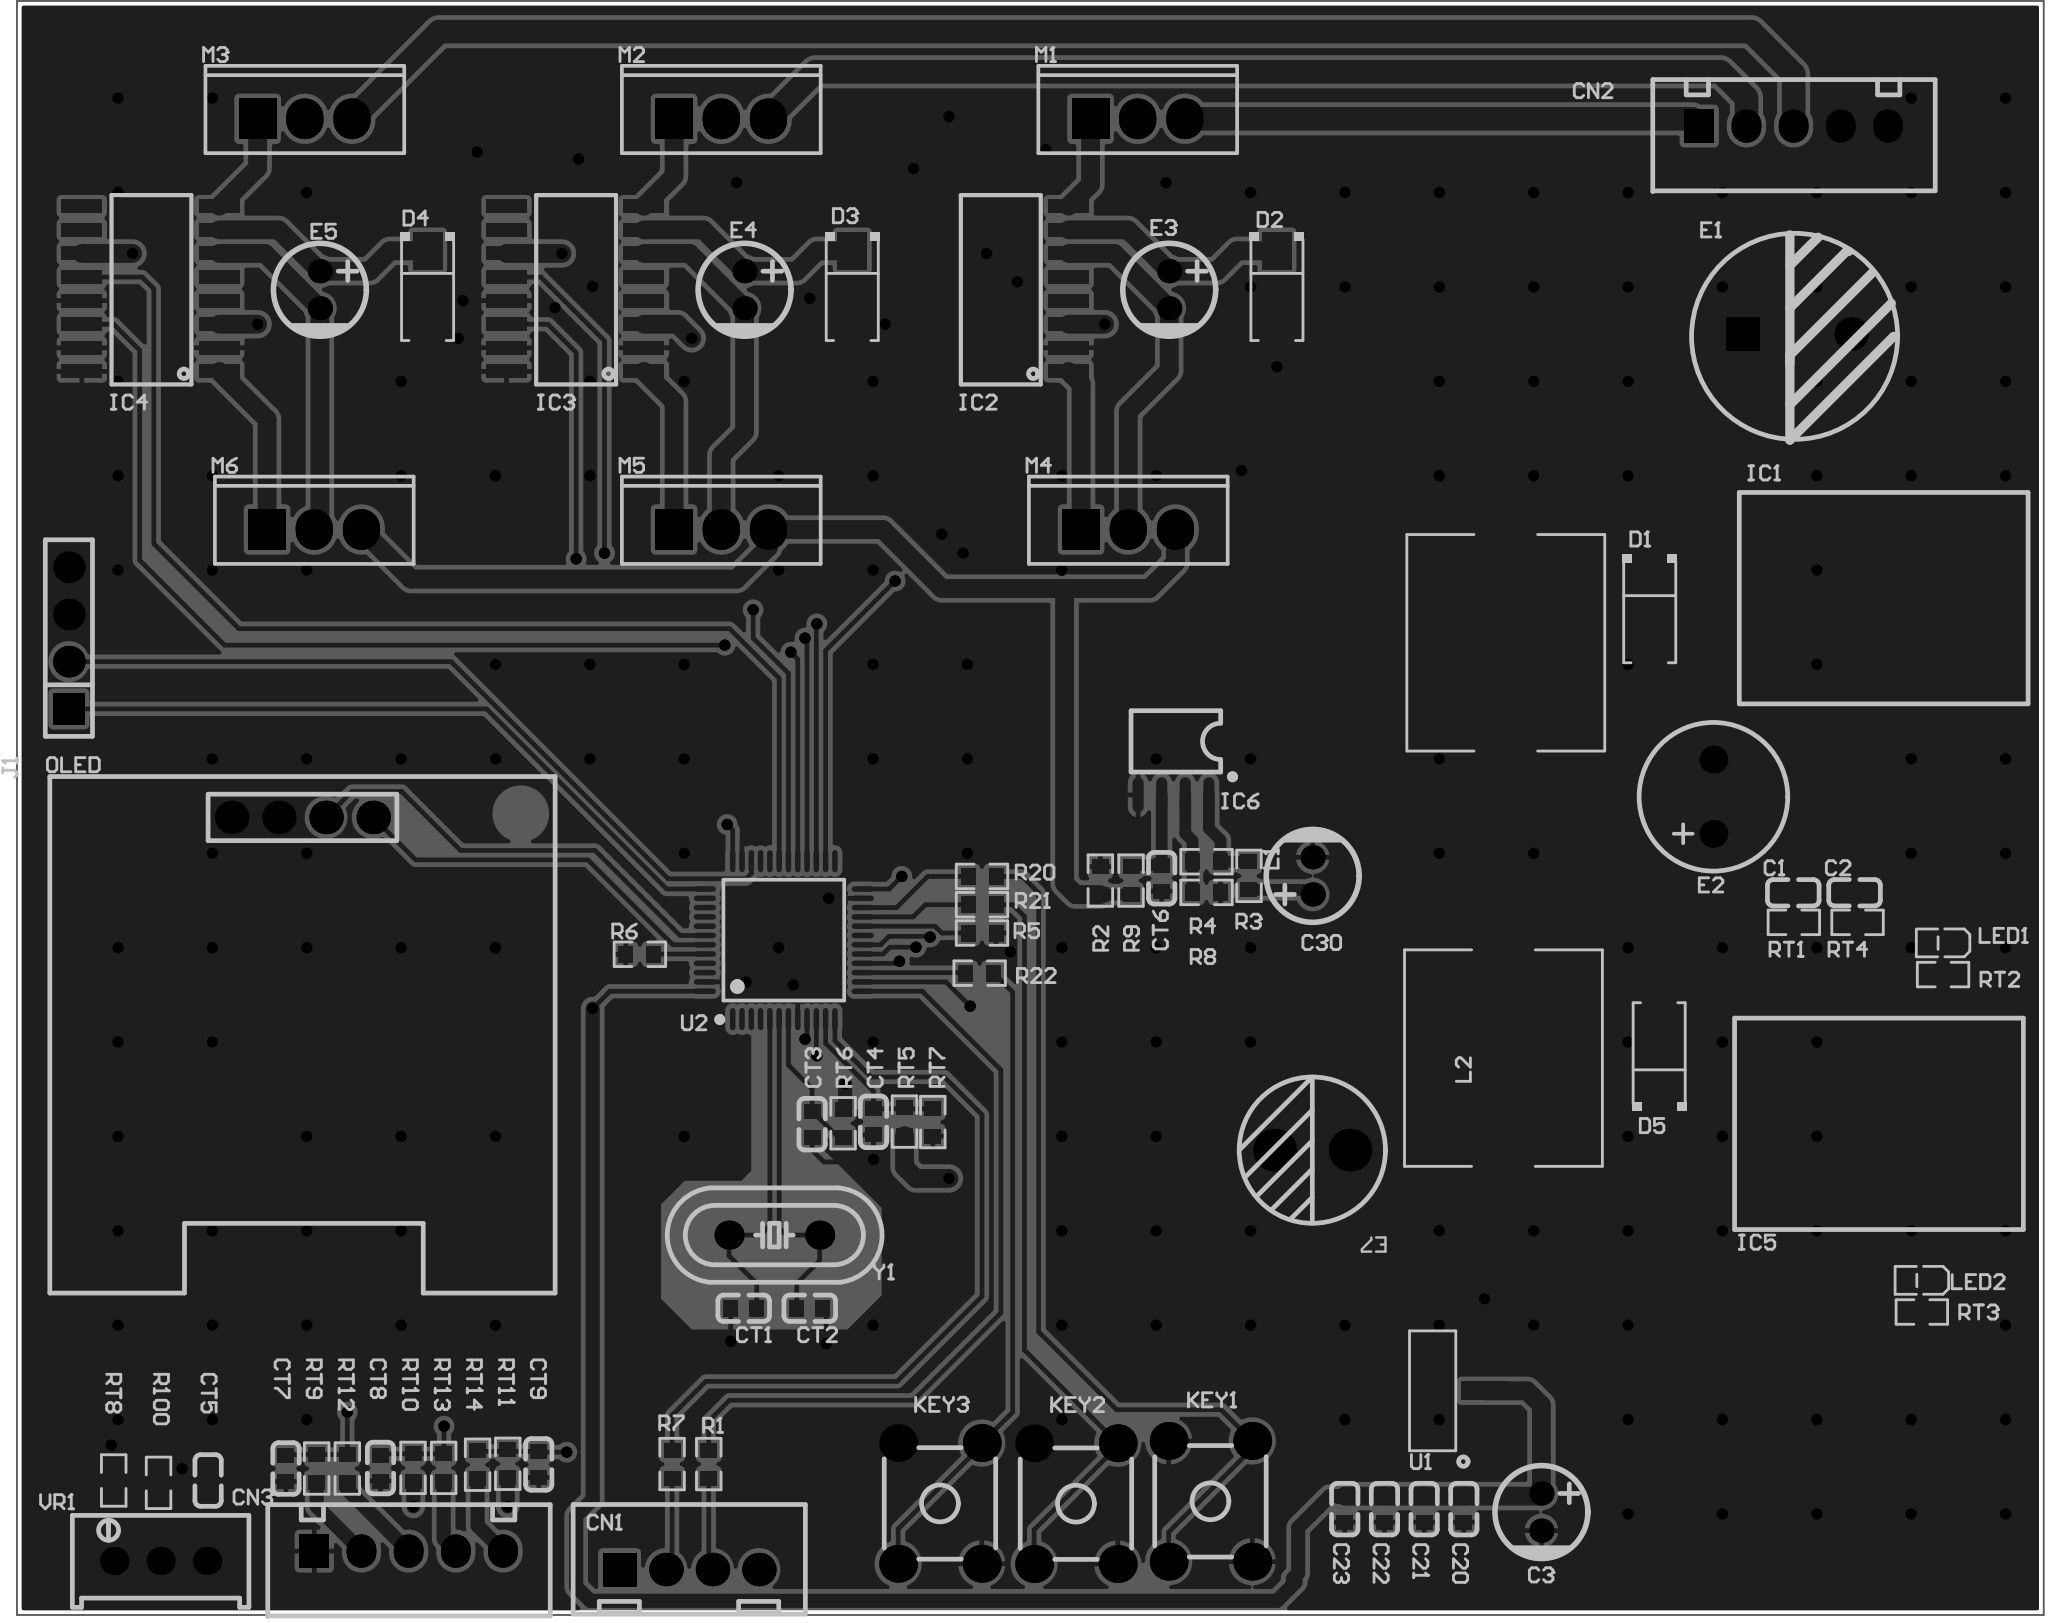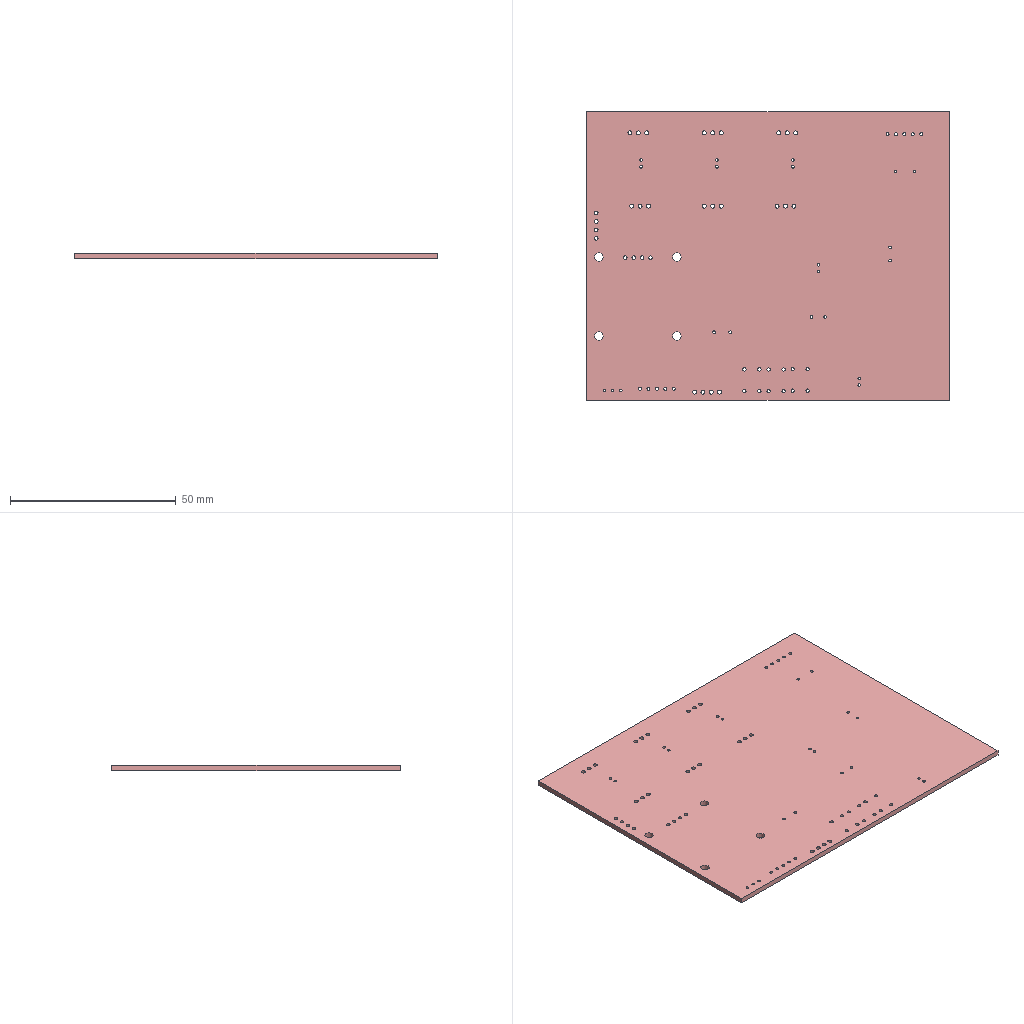Circuit board layout | Altium Designer | box 109.1 x 86.9 x 1.6 mm
Layer stack:
# Altium Designer layer stack of  (unit mm; dielectric type: 0 none, 1 core, 2 prepreg, 3 surface material)
index,name,kind,layer,copper_thickness_mm,dielectric_type,dielectric_thickness_mm,dielectric_material,dielectric_constant
0,Top Paste Mask Layer,other,,,,,,
1,Top Silkscreen Layer,other,,,,,,
2,Top Solder Mask Layer,dielectric,,,3,0.01,,3.3
3,Top Layer,copper,Top Layer,0.035,,,,
4,Dielectric1,dielectric,,,3,1.51,FR4,4.5
5,Bottom Layer,copper,Bottom Layer,0.035,,,,
6,Bottom Solder Mask Layer,dielectric,,,3,0.01,,3.3
7,Bottom Silkscreen Layer,other,,,,,,
8,Bottom Paste Mask Layer,other,,,,,,
# drill layer pairs: low layer,high layer
drill_pair,Top Layer,Bottom Layer
Part placement:
Designator,Comment,Layer,Footprint,Center-X(mm),Center-Y(mm),Rotation
C1,104,TopLayer,C0603,184.637,125.864,0
C2,104,TopLayer,C0603,187.936,125.867,0
C3,16V/220uF,TopLayer,CAP-TH_BD5.0-P2.00-D0.8-FD-10UF50VC110GL,171.082,92.536,270
C20,104,TopLayer,C0603,166.906,92.693,270
C21,104,TopLayer,C0603,164.769,92.693,270
C22,104,TopLayer,C0603,162.632,92.693,270
C23,104,TopLayer,C0603,160.495,92.693,270
C30,106,TopLayer,CAP-TH_BD5.0-P2.00-D0.8-FD-10UF50VC110GL,158.77,126.775,90
CT1,30pf,TopLayer,C0603,128.143,103.505,180
CT2,30pf,TopLayer,C0603,131.699,103.505,180
CT3,105,TopLayer,C0603,131.826,113.411,90
CT4,104,TopLayer,C0603,135.128,113.538,90
CT5,104,TopLayer,C0603,99.314,94.234,90
CT6,104,TopLayer,C0603,150.642,126.648,90
CT7,104,TopLayer,C0603,103.506,94.879,90
CT8,104,TopLayer,C0603,108.594,94.906,90
CT9,104,TopLayer,C0603,117.11,95.098,90
D1,SS34/1N5822,TopLayer,SMA_L4.3-W2.5-LS5.0-RD,176.911,140.97,270
D2,M4,TopLayer,SMA_L4.3-W2.5-LS5.0-RD,156.845,158.314,270
D3,M4,TopLayer,SMA_L4.3-W2.5-LS5.0-RD,133.987,158.314,270
D4,M4,TopLayer,SMA_L4.3-W2.5-LS5.0-RD,111.129,158.314,270
D5,SS34/1N5822,TopLayer,SMA_L4.3-W2.5-LS5.0-RD,177.419,117.221,90
E1,50V/330uF,TopLayer,50v/330uf,184.835,155.94,0
E2,50V/100uF,TopLayer,50V/100UF,180.34,131.032,90
E3,10UF,TopLayer,CAP-TH_BD5.0-P2.00-D0.8-FD-10UF50VC110GL,151.048,158.319,270
E4,10UF,TopLayer,CAP-TH_BD5.0-P2.00-D0.8-FD-10UF50VC110GL,128.19,158.319,270
E5,10UF,TopLayer,CAP-TH_BD5.0-P2.00-D0.8-FD-10UF50VC110GL,105.332,158.319,270
E7,16V/220uF,TopLayer,16V/220UF,158.75,112.014,180
IC1,LM2596S,TopLayer,LM2596S,187.599,141.695,270
IC2,IR2113S,TopLayer,SOP-16,141.933,158.369,90
IC3,IR2113S,TopLayer,SOP-16,119.074,158.369,90
IC4,IR2113S,TopLayer,SOP-16,96.216,158.369,90
IC5,LM2596S-5V,TopLayer,LM2596S,187.345,113.404,270
IC6,LM358,TopLayer,lm358,151.277,134.035,180
KEY1,,TopLayer,SW-PB1,153.266,93.114,270
KEY2,,TopLayer,SW-PB1,146.027,92.987,270
KEY3,,TopLayer,SW-PB1,138.707,93,270
M1,IR540,TopLayer,IR5401,149.352,167.521,0
M2,IR540,TopLayer,IR5401,126.936,167.521,0
M3,IR540,TopLayer,IR5401,104.521,167.521,0
M4,IR540,TopLayer,IR5401,148.844,145.415,0
M5,IR540,TopLayer,IR5401,126.936,145.415,0
M6,IR540,TopLayer,IR5401,105.029,145.415,0
OLED,OLED,TopLayer,OLED,104.394,129.921,0
R1,100R,TopLayer,R0603,126.263,95.118,90
R2,0.22R,TopLayer,R0603,147.34,126.521,90
R3,1K,TopLayer,R0603,155.341,126.775,90
R4,10K,TopLayer,R0603,153.055,127.537,0
R5,4.7K,TopLayer,R0603,140.97,123.698,180
R6,4.7K,TopLayer,R0603,122.555,122.555,0
R7,100R,TopLayer,R0603,124.289,95.118,90
R8,1K,TopLayer,R0603,153.055,125.886,0
R9,1K,TopLayer,R0603,148.991,126.521,90
R20,10K,TopLayer,R0603,140.97,126.746,0
R21,10K,TopLayer,R0603,140.97,125.222,0
R22,10K,TopLayer,R0603,140.843,121.539,0
R100,1K,TopLayer,R0603,96.647,94.107,270
RT1,10K,TopLayer,R0603,184.669,124.273,180
RT2,1K,TopLayer,R0603,192.701,121.463,180
RT3,1K,TopLayer,R0603,191.558,103.302,180
RT4,1K,TopLayer,R0603,188.098,124.273,180
RT5,20K,TopLayer,R0603,136.798,113.55,270
RT6,10K,TopLayer,R0603,133.494,113.459,90
RT7,1K,TopLayer,R0603,138.322,113.526,90
RT8,5K,TopLayer,R0603,94.234,94.234,90
RT9,10K,TopLayer,R0603,105.157,94.879,270
RT10,10K,TopLayer,R0603,110.344,94.913,270
RT11,10K,TopLayer,R0603,115.444,95.132,270
RT12,220R,TopLayer,R0603,106.808,94.879,270
RT13,220R,TopLayer,R0603,111.995,94.913,270
RT14,220R,TopLayer,R0603,113.821,95.083,270
U1,1117-3.3V,TopLayer,1117-3.3V,165.227,99.06,180
U2,STM32F103C8T6,TopLayer,STM32F103C8T6,130.302,123.317,90
VR1,10K,TopLayer,R_3296,96.757,89.904,0
Y1,8M,TopLayer,HC-49S_L11.5-W5.0-P4.88,129.794,107.442,180
CN1,CON4,TopLayer,CON4,125.213,89.441,0
CN2,CON5,TopLayer,CON5,184.658,167.132,0
CN3,CON5,TopLayer,CON5,110.11,90.433,0
LED1,REG,TopLayer,LED0603,192.651,123.173,180
LED2,REG,TopLayer,LED0603,191.508,105.012,180
J1,CON4(NC),TopLayer,HDR-TH_4P-P2.54-V-F,91.821,139.573,90
L1,33UH/3A,TopLayer,IND-SMD_L11.5-W10.5_MWSA1004,169.164,139.319,90
L2,33UH/3A,TopLayer,IND-SMD_L11.5-W10.5_MWSA1004,169.037,116.967,90
Pad and via stacks:
# Altium Designer via and pad stacks of  (unit mm). Each distinct definition once, with the count of objects using it.
# via: kind,start_layer,end_layer,hole_mm,diameter_mm,mode(0 simple;1 top-mid-bottom;2 full stack),diameter_per_layer,count,example_net
# pad: kind,layer,hole_mm,hole_type(0 round;1 square;2 slot),plating,top_size,top_shape(1 round;2 rect;3 octagon;9 rounded rect),mid_size,bottom_size,mode,footprint,size_per_layer,count,example
pad,Top Layer,0,0,plated,0.8x0.9,2,0.8x0.9,0.8x0.9,0,C0603,,30,C1.2
pad,Top Layer,0,0,plated,2x1.593,2,2x1.593,2x1.593,0,SMA_L4.3-W2.5-LS5.0-RD,,10,D1.2
pad,Top Layer,0,0,plated,10.414x10.82,2,10.414x10.82,10.414x10.82,0,LM2596S,,2,IC1.3
pad,Top Layer,0,0,plated,2.54x1.067,2,2.54x1.067,2.54x1.067,0,LM2596S,,10,IC1.3
pad,Top Layer,0,0,plated,0.701x2.2,2,0.701x2.2,0.701x2.2,0,SOP-16,,48,IC2.1
pad,Top Layer,0,0,plated,0.6x1.9,1,0.6x1.9,0.6x1.9,0,lm358,,8,IC6.1
pad,Top Layer,0,0,plated,0.8065x0.864,2,0.8065x0.864,0.8065x0.864,0,R0603,,54,R1.2
pad,Top Layer,0,0,plated,2.565x1.015,2,2.565x1.015,2.565x1.015,0,1117-3.3V,,3,U1.1
pad,Top Layer,0,0,plated,2.565x3.6,2,2.565x3.6,2.565x3.6,0,1117-3.3V,,1,U1.4
pad,Top Layer,0,0,plated,0.2997x1.199,1,0.2997x1.199,0.2997x1.199,0,STM32F103C8T6,,48,U2.1
pad,Top Layer,0,0,plated,0.8x0.8,2,0.8x0.8,0.8x0.8,0,LED0603,,4,LED1.2
pad,Top Layer,0,0,plated,3.424x3.12,2,3.424x3.12,3.424x3.12,0,IND-SMD_L11.5-W10.5_MWSA1004,,4,L1.1
pad,Multi-Layer,0.8,0,plated,1.3x1.3,1,1.3x1.3,1.3x1.3,0,CAP-TH_BD5.0-P2.00-D0.8-FD-10UF50VC110GL,,10,C3.2
pad,Multi-Layer,0.762,0,plated,1.8x1.8,2,1.8x1.8,1.8x1.8,0,50v/330uf,,1,E1.1
pad,Multi-Layer,0.762,0,plated,1.8x1.8,1,1.8x1.8,1.8x1.8,0,50v/330uf,,1,E1.2
pad,Multi-Layer,0.8,0,plated,1.5x1.5,1,1.5x1.5,1.5x1.5,0,50V/100UF,,2,E2.1
pad,Multi-Layer,0.8128,0,plated,2.3x2.3,1,2.3x2.3,2.3x2.3,0,16V/220UF,,2,E7.1
pad,Multi-Layer,1.016,0,plated,2.032x2.032,1,2.032x2.032,2.032x2.032,0,SW-PB1,,12,KEY1.1
pad,Multi-Layer,1.2,0,plated,2x2.2,1,2x2.2,2x2.2,0,IR5401,,12,M1.3
pad,Multi-Layer,1.2,0,plated,2x2.2,2,2x2.2,2x2.2,0,IR5401,,6,M1.1
pad,Multi-Layer,1.05,0,plated,1.8x1.8,1,1.8x1.8,1.8x1.8,0,OLED,,4,OLED.1
pad,Multi-Layer,0.762,0,plated,1.524x1.524,1,1.524x1.524,1.524x1.524,0,R_3296,,3,VR1.2
pad,Multi-Layer,0.9,0,plated,1.56x1.56,1,1.56x1.56,1.56x1.56,0,HC-49S_L11.5-W5.0-P4.88,,2,Y1.1
pad,Multi-Layer,1.2,0,plated,1.8x1.8,2,1.8x1.8,1.8x1.8,0,CON4,,1,CN1.1
pad,Multi-Layer,1.2,0,plated,1.8x1.8,1,1.8x1.8,1.8x1.8,0,CON4,,3,CN1.2
pad,Multi-Layer,0.9,0,plated,1.6x1.8,2,1.6x1.8,1.6x1.8,0,CON5,,2,CN2.1
pad,Multi-Layer,0.9,0,plated,1.6x1.8,1,1.6x1.8,1.6x1.8,0,CON5,,8,CN2.2
pad,Multi-Layer,1.1,0,plated,1.7x1.7,2,1.7x1.7,1.7x1.7,0,HDR-TH_4P-P2.54-V-F,,1,J1.1
pad,Multi-Layer,1.1,0,plated,1.7x1.7,1,1.7x1.7,1.7x1.7,0,HDR-TH_4P-P2.54-V-F,,3,J1.2
via,Top Layer,Bottom Layer,0.3048,0.61,0,,220,PB0
Copper pours:
name,layer,net,type(0 solid;1 hatched;2 none)
Top Layer-GND,Top Layer,GND,0
Bottom Layer-GND,Bottom Layer,GND,0
Design rules, without the lines most boards share:
# Altium Designer design rules of  (exported by Altium Designer, unit mm)
# columns: name | kind | enabled | priority | scope1 | scope2 | descriptor | typed fields (field=value)
creepage | 65 | enabled | 1 | All | All | Creepage Distance Constraint =(0mil) (All),(All) |